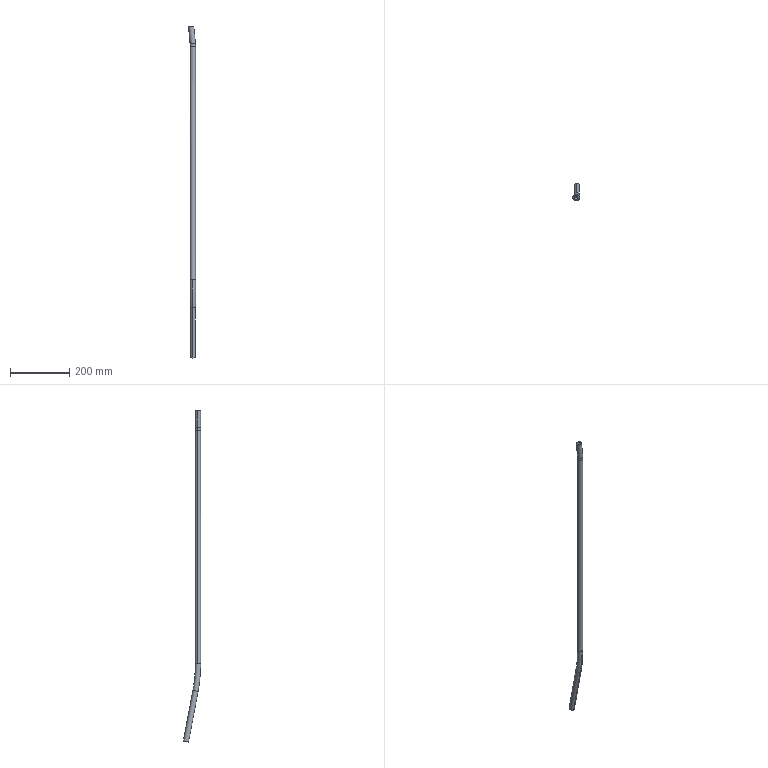Part | STEP file | Lower Chain Tube | 1 solid | 22 faces | box 23.853 x 58.527 x 1125 mm | volume 60168 mm3 | cylinder 12 | torus 8 | plane 2 | commonest cylinder face diameters 16 x6 18 x6
STEP:
#1=CARTESIAN_POINT('',(0.,0.,0.));
#2=DIRECTION('',(0.,0.,1.));
#3=DIRECTION('',(1.,0.,0.));
#4=AXIS2_PLACEMENT_3D('',#1,#2,#3);
#5=CARTESIAN_POINT('',(-8.,0.,3.704));
#6=VERTEX_POINT('',#5);
#7=CARTESIAN_POINT('',(-8.41,0.,12.377));
#8=VERTEX_POINT('',#7);
#9=CARTESIAN_POINT('',(-100.,0.,3.704));
#10=DIRECTION('',(0.,-1.,0.));
#11=DIRECTION('',(0.,0.,-1.));
#12=AXIS2_PLACEMENT_3D('',#9,#10,#11);
#13=CIRCLE('',#12,92.);
#14=CARTESIAN_POINT('',(-100.,0.,3.704));
#15=DIRECTION('',(0.,-1.,0.));
#16=DIRECTION('',(0.,0.,-1.));
#17=AXIS2_PLACEMENT_3D('',#14,#15,#16);
#18=TOROIDAL_SURFACE('',#17,100.,8.);
#19=CARTESIAN_POINT('',(0.,3.142));
#20=DIRECTION('',(1.,0.));
#21=VECTOR('',#20,1.);
#22=LINE('',#19,#21);
#23=(GEOMETRIC_REPRESENTATION_CONTEXT(2)PARAMETRIC_REPRESENTATION_CONTEXT()REPRESENTATION_CONTEXT('',''));
#24=DEFINITIONAL_REPRESENTATION('',(#22),#23);
#25=PCURVE('',#18,#24);
#26=CARTESIAN_POINT('',(-100.,0.,3.704));
#27=DIRECTION('',(0.,-1.,0.));
#28=DIRECTION('',(0.,0.,-1.));
#29=AXIS2_PLACEMENT_3D('',#26,#27,#28);
#30=TOROIDAL_SURFACE('',#29,100.,8.);
#31=CARTESIAN_POINT('',(0.,3.142));
#32=DIRECTION('',(1.,0.));
#33=VECTOR('',#32,1.);
#34=LINE('',#31,#33);
#35=(GEOMETRIC_REPRESENTATION_CONTEXT(2)PARAMETRIC_REPRESENTATION_CONTEXT()REPRESENTATION_CONTEXT('',''));
#36=DEFINITIONAL_REPRESENTATION('',(#34),#35);
#37=PCURVE('',#30,#36);
#38=SURFACE_CURVE('',#13,(#25,#37),.PCURVE_S1.);
#39=EDGE_CURVE('',#6,#8,#38,.T.);
#40=ORIENTED_EDGE('',*,*,#39,.T.);
#41=CARTESIAN_POINT('',(7.519,0.,13.885));
#42=VERTEX_POINT('',#41);
#43=CARTESIAN_POINT('',(-0.4454,0.,13.131));
#44=DIRECTION('',(-0.09427,0.,0.9955));
#45=DIRECTION('',(0.9955,0.,0.09427));
#46=AXIS2_PLACEMENT_3D('',#43,#44,#45);
#47=CIRCLE('',#46,8.);
#48=CARTESIAN_POINT('',(1.665,6.283));
#49=DIRECTION('',(0.,-1.));
#50=VECTOR('',#49,1.);
#51=LINE('',#48,#50);
#52=(GEOMETRIC_REPRESENTATION_CONTEXT(2)PARAMETRIC_REPRESENTATION_CONTEXT()REPRESENTATION_CONTEXT('',''));
#53=DEFINITIONAL_REPRESENTATION('',(#51),#52);
#54=PCURVE('',#18,#53);
#55=CARTESIAN_POINT('',(-0.4454,0.,13.131));
#56=DIRECTION('',(-0.09427,0.,0.9955));
#57=DIRECTION('',(0.9955,0.,0.09427));
#58=AXIS2_PLACEMENT_3D('',#55,#56,#57);
#59=CYLINDRICAL_SURFACE('',#58,8.);
#60=CARTESIAN_POINT('',(0.,0.));
#61=DIRECTION('',(1.,0.));
#62=VECTOR('',#61,1.);
#63=LINE('',#60,#62);
#64=(GEOMETRIC_REPRESENTATION_CONTEXT(2)PARAMETRIC_REPRESENTATION_CONTEXT()REPRESENTATION_CONTEXT('',''));
#65=DEFINITIONAL_REPRESENTATION('',(#63),#64);
#66=PCURVE('',#59,#65);
#67=SURFACE_CURVE('',#47,(#54,#66),.PCURVE_S1.);
#68=EDGE_CURVE('',#42,#8,#67,.T.);
#69=ORIENTED_EDGE('',*,*,#68,.F.);
#70=CARTESIAN_POINT('',(8.,0.,3.704));
#71=VERTEX_POINT('',#70);
#72=CARTESIAN_POINT('',(-100.,0.,3.704));
#73=DIRECTION('',(0.,-1.,0.));
#74=DIRECTION('',(0.,0.,-1.));
#75=AXIS2_PLACEMENT_3D('',#72,#73,#74);
#76=CIRCLE('',#75,108.);
#77=CARTESIAN_POINT('',(0.,6.283));
#78=DIRECTION('',(1.,0.));
#79=VECTOR('',#78,1.);
#80=LINE('',#77,#79);
#81=(GEOMETRIC_REPRESENTATION_CONTEXT(2)PARAMETRIC_REPRESENTATION_CONTEXT()REPRESENTATION_CONTEXT('',''));
#82=DEFINITIONAL_REPRESENTATION('',(#80),#81);
#83=PCURVE('',#18,#82);
#84=CARTESIAN_POINT('',(0.,0.));
#85=DIRECTION('',(1.,0.));
#86=VECTOR('',#85,1.);
#87=LINE('',#84,#86);
#88=(GEOMETRIC_REPRESENTATION_CONTEXT(2)PARAMETRIC_REPRESENTATION_CONTEXT()REPRESENTATION_CONTEXT('',''));
#89=DEFINITIONAL_REPRESENTATION('',(#87),#88);
#90=PCURVE('',#30,#89);
#91=SURFACE_CURVE('',#76,(#83,#90),.PCURVE_S1.);
#92=EDGE_CURVE('',#71,#42,#91,.T.);
#93=ORIENTED_EDGE('',*,*,#92,.F.);
#94=CARTESIAN_POINT('',(0.,0.,3.704));
#95=DIRECTION('',(0.,0.,1.));
#96=DIRECTION('',(1.,0.,0.));
#97=AXIS2_PLACEMENT_3D('',#94,#95,#96);
#98=CIRCLE('',#97,8.);
#99=CARTESIAN_POINT('',(1.571,6.283));
#100=DIRECTION('',(0.,-1.));
#101=VECTOR('',#100,1.);
#102=LINE('',#99,#101);
#103=(GEOMETRIC_REPRESENTATION_CONTEXT(2)PARAMETRIC_REPRESENTATION_CONTEXT()REPRESENTATION_CONTEXT('',''));
#104=DEFINITIONAL_REPRESENTATION('',(#102),#103);
#105=PCURVE('',#18,#104);
#106=CARTESIAN_POINT('',(0.,0.,-788.57));
#107=DIRECTION('',(0.,0.,1.));
#108=DIRECTION('',(1.,0.,0.));
#109=AXIS2_PLACEMENT_3D('',#106,#107,#108);
#110=CYLINDRICAL_SURFACE('',#109,8.);
#111=CARTESIAN_POINT('',(0.,792.273));
#112=DIRECTION('',(1.,0.));
#113=VECTOR('',#112,1.);
#114=LINE('',#111,#113);
#115=(GEOMETRIC_REPRESENTATION_CONTEXT(2)PARAMETRIC_REPRESENTATION_CONTEXT()REPRESENTATION_CONTEXT('',''));
#116=DEFINITIONAL_REPRESENTATION('',(#114),#115);
#117=PCURVE('',#110,#116);
#118=SURFACE_CURVE('',#98,(#105,#117),.PCURVE_S1.);
#119=EDGE_CURVE('',#71,#6,#118,.T.);
#120=ORIENTED_EDGE('',*,*,#119,.T.);
#121=EDGE_LOOP('',(#40,#69,#93,#120));
#122=FACE_BOUND('',#121,.F.);
#123=ADVANCED_FACE('',(#122),#18,.F.);
#124=CARTESIAN_POINT('',(-9.,0.,3.704));
#125=VERTEX_POINT('',#124);
#126=CARTESIAN_POINT('',(9.,0.,3.704));
#127=VERTEX_POINT('',#126);
#128=CARTESIAN_POINT('',(0.,0.,3.704));
#129=DIRECTION('',(0.,0.,1.));
#130=DIRECTION('',(1.,0.,0.));
#131=AXIS2_PLACEMENT_3D('',#128,#129,#130);
#132=CIRCLE('',#131,9.);
#133=CARTESIAN_POINT('',(-100.,0.,3.704));
#134=DIRECTION('',(0.,-1.,0.));
#135=DIRECTION('',(0.,0.,-1.));
#136=AXIS2_PLACEMENT_3D('',#133,#134,#135);
#137=TOROIDAL_SURFACE('',#136,100.,9.);
#138=CARTESIAN_POINT('',(1.571,6.283));
#139=DIRECTION('',(0.,-1.));
#140=VECTOR('',#139,1.);
#141=LINE('',#138,#140);
#142=(GEOMETRIC_REPRESENTATION_CONTEXT(2)PARAMETRIC_REPRESENTATION_CONTEXT()REPRESENTATION_CONTEXT('',''));
#143=DEFINITIONAL_REPRESENTATION('',(#141),#142);
#144=PCURVE('',#137,#143);
#145=CARTESIAN_POINT('',(0.,0.,-788.57));
#146=DIRECTION('',(0.,0.,1.));
#147=DIRECTION('',(1.,0.,0.));
#148=AXIS2_PLACEMENT_3D('',#145,#146,#147);
#149=CYLINDRICAL_SURFACE('',#148,9.);
#150=CARTESIAN_POINT('',(0.,792.273));
#151=DIRECTION('',(1.,0.));
#152=VECTOR('',#151,1.);
#153=LINE('',#150,#152);
#154=(GEOMETRIC_REPRESENTATION_CONTEXT(2)PARAMETRIC_REPRESENTATION_CONTEXT()REPRESENTATION_CONTEXT('',''));
#155=DEFINITIONAL_REPRESENTATION('',(#153),#154);
#156=PCURVE('',#149,#155);
#157=SURFACE_CURVE('',#132,(#144,#156),.PCURVE_S1.);
#158=EDGE_CURVE('',#125,#127,#157,.T.);
#159=ORIENTED_EDGE('',*,*,#158,.T.);
#160=CARTESIAN_POINT('',(8.515,0.,13.979));
#161=VERTEX_POINT('',#160);
#162=CARTESIAN_POINT('',(-100.,0.,3.704));
#163=DIRECTION('',(0.,-1.,0.));
#164=DIRECTION('',(0.,0.,-1.));
#165=AXIS2_PLACEMENT_3D('',#162,#163,#164);
#166=CIRCLE('',#165,109.);
#167=CARTESIAN_POINT('',(0.,0.));
#168=DIRECTION('',(1.,0.));
#169=VECTOR('',#168,1.);
#170=LINE('',#167,#169);
#171=(GEOMETRIC_REPRESENTATION_CONTEXT(2)PARAMETRIC_REPRESENTATION_CONTEXT()REPRESENTATION_CONTEXT('',''));
#172=DEFINITIONAL_REPRESENTATION('',(#170),#171);
#173=PCURVE('',#137,#172);
#174=CARTESIAN_POINT('',(-100.,0.,3.704));
#175=DIRECTION('',(0.,-1.,0.));
#176=DIRECTION('',(0.,0.,-1.));
#177=AXIS2_PLACEMENT_3D('',#174,#175,#176);
#178=TOROIDAL_SURFACE('',#177,100.,9.);
#179=CARTESIAN_POINT('',(0.,6.283));
#180=DIRECTION('',(1.,0.));
#181=VECTOR('',#180,1.);
#182=LINE('',#179,#181);
#183=(GEOMETRIC_REPRESENTATION_CONTEXT(2)PARAMETRIC_REPRESENTATION_CONTEXT()REPRESENTATION_CONTEXT('',''));
#184=DEFINITIONAL_REPRESENTATION('',(#182),#183);
#185=PCURVE('',#178,#184);
#186=SURFACE_CURVE('',#166,(#173,#185),.PCURVE_S1.);
#187=EDGE_CURVE('',#127,#161,#186,.T.);
#188=ORIENTED_EDGE('',*,*,#187,.T.);
#189=CARTESIAN_POINT('',(-9.405,0.,12.283));
#190=VERTEX_POINT('',#189);
#191=CARTESIAN_POINT('',(-0.4454,0.,13.131));
#192=DIRECTION('',(-0.09427,0.,0.9955));
#193=DIRECTION('',(0.9955,0.,0.09427));
#194=AXIS2_PLACEMENT_3D('',#191,#192,#193);
#195=CIRCLE('',#194,9.);
#196=CARTESIAN_POINT('',(1.665,6.283));
#197=DIRECTION('',(0.,-1.));
#198=VECTOR('',#197,1.);
#199=LINE('',#196,#198);
#200=(GEOMETRIC_REPRESENTATION_CONTEXT(2)PARAMETRIC_REPRESENTATION_CONTEXT()REPRESENTATION_CONTEXT('',''));
#201=DEFINITIONAL_REPRESENTATION('',(#199),#200);
#202=PCURVE('',#137,#201);
#203=CARTESIAN_POINT('',(-0.4454,0.,13.131));
#204=DIRECTION('',(-0.09427,0.,0.9955));
#205=DIRECTION('',(0.9955,0.,0.09427));
#206=AXIS2_PLACEMENT_3D('',#203,#204,#205);
#207=CYLINDRICAL_SURFACE('',#206,9.);
#208=CARTESIAN_POINT('',(0.,0.));
#209=DIRECTION('',(1.,0.));
#210=VECTOR('',#209,1.);
#211=LINE('',#208,#210);
#212=(GEOMETRIC_REPRESENTATION_CONTEXT(2)PARAMETRIC_REPRESENTATION_CONTEXT()REPRESENTATION_CONTEXT('',''));
#213=DEFINITIONAL_REPRESENTATION('',(#211),#212);
#214=PCURVE('',#207,#213);
#215=SURFACE_CURVE('',#195,(#202,#214),.PCURVE_S1.);
#216=EDGE_CURVE('',#190,#161,#215,.T.);
#217=ORIENTED_EDGE('',*,*,#216,.F.);
#218=CARTESIAN_POINT('',(-100.,0.,3.704));
#219=DIRECTION('',(0.,-1.,0.));
#220=DIRECTION('',(0.,0.,-1.));
#221=AXIS2_PLACEMENT_3D('',#218,#219,#220);
#222=CIRCLE('',#221,91.);
#223=CARTESIAN_POINT('',(0.,3.142));
#224=DIRECTION('',(1.,0.));
#225=VECTOR('',#224,1.);
#226=LINE('',#223,#225);
#227=(GEOMETRIC_REPRESENTATION_CONTEXT(2)PARAMETRIC_REPRESENTATION_CONTEXT()REPRESENTATION_CONTEXT('',''));
#228=DEFINITIONAL_REPRESENTATION('',(#226),#227);
#229=PCURVE('',#137,#228);
#230=CARTESIAN_POINT('',(0.,3.142));
#231=DIRECTION('',(1.,0.));
#232=VECTOR('',#231,1.);
#233=LINE('',#230,#232);
#234=(GEOMETRIC_REPRESENTATION_CONTEXT(2)PARAMETRIC_REPRESENTATION_CONTEXT()REPRESENTATION_CONTEXT('',''));
#235=DEFINITIONAL_REPRESENTATION('',(#233),#234);
#236=PCURVE('',#178,#235);
#237=SURFACE_CURVE('',#222,(#229,#236),.PCURVE_S1.);
#238=EDGE_CURVE('',#125,#190,#237,.T.);
#239=ORIENTED_EDGE('',*,*,#238,.F.);
#240=EDGE_LOOP('',(#159,#188,#217,#239));
#241=FACE_BOUND('',#240,.T.);
#242=ADVANCED_FACE('',(#241),#137,.T.);
#243=CARTESIAN_POINT('',(0.,8.,-788.57));
#244=VERTEX_POINT('',#243);
#245=CARTESIAN_POINT('',(-8.,0.,-788.57));
#246=VERTEX_POINT('',#245);
#247=CARTESIAN_POINT('',(0.,0.,-788.57));
#248=DIRECTION('',(0.,0.,1.));
#249=DIRECTION('',(1.,0.,0.));
#250=AXIS2_PLACEMENT_3D('',#247,#248,#249);
#251=CIRCLE('',#250,8.);
#252=CARTESIAN_POINT('',(0.,500.,-788.57));
#253=DIRECTION('',(1.,0.,0.));
#254=DIRECTION('',(0.,0.,-1.));
#255=AXIS2_PLACEMENT_3D('',#252,#253,#254);
#256=TOROIDAL_SURFACE('',#255,500.,8.);
#257=CARTESIAN_POINT('',(4.712,1.571));
#258=DIRECTION('',(0.,1.));
#259=VECTOR('',#258,1.);
#260=LINE('',#257,#259);
#261=(GEOMETRIC_REPRESENTATION_CONTEXT(2)PARAMETRIC_REPRESENTATION_CONTEXT()REPRESENTATION_CONTEXT('',''));
#262=DEFINITIONAL_REPRESENTATION('',(#260),#261);
#263=PCURVE('',#256,#262);
#264=CARTESIAN_POINT('',(0.,0.));
#265=DIRECTION('',(1.,0.));
#266=VECTOR('',#265,1.);
#267=LINE('',#264,#266);
#268=(GEOMETRIC_REPRESENTATION_CONTEXT(2)PARAMETRIC_REPRESENTATION_CONTEXT()REPRESENTATION_CONTEXT('',''));
#269=DEFINITIONAL_REPRESENTATION('',(#267),#268);
#270=PCURVE('',#110,#269);
#271=SURFACE_CURVE('',#251,(#263,#270),.PCURVE_S1.);
#272=EDGE_CURVE('',#244,#246,#271,.T.);
#273=ORIENTED_EDGE('',*,*,#272,.F.);
#274=CARTESIAN_POINT('',(0.,16.413,-879.163));
#275=VERTEX_POINT('',#274);
#276=CARTESIAN_POINT('',(0.,500.,-788.57));
#277=DIRECTION('',(1.,0.,0.));
#278=DIRECTION('',(0.,0.,-1.));
#279=AXIS2_PLACEMENT_3D('',#276,#277,#278);
#280=CIRCLE('',#279,492.);
#281=CARTESIAN_POINT('',(0.,3.142));
#282=DIRECTION('',(1.,0.));
#283=VECTOR('',#282,1.);
#284=LINE('',#281,#283);
#285=(GEOMETRIC_REPRESENTATION_CONTEXT(2)PARAMETRIC_REPRESENTATION_CONTEXT()REPRESENTATION_CONTEXT('',''));
#286=DEFINITIONAL_REPRESENTATION('',(#284),#285);
#287=PCURVE('',#256,#286);
#288=CARTESIAN_POINT('',(0.,500.,-788.57));
#289=DIRECTION('',(1.,0.,0.));
#290=DIRECTION('',(0.,0.,-1.));
#291=AXIS2_PLACEMENT_3D('',#288,#289,#290);
#292=TOROIDAL_SURFACE('',#291,500.,8.);
#293=CARTESIAN_POINT('',(0.,3.142));
#294=DIRECTION('',(1.,0.));
#295=VECTOR('',#294,1.);
#296=LINE('',#293,#295);
#297=(GEOMETRIC_REPRESENTATION_CONTEXT(2)PARAMETRIC_REPRESENTATION_CONTEXT()REPRESENTATION_CONTEXT('',''));
#298=DEFINITIONAL_REPRESENTATION('',(#296),#297);
#299=PCURVE('',#292,#298);
#300=SURFACE_CURVE('',#280,(#287,#299),.PCURVE_S1.);
#301=EDGE_CURVE('',#244,#275,#300,.T.);
#302=ORIENTED_EDGE('',*,*,#301,.T.);
#303=CARTESIAN_POINT('',(0.,0.6862,-882.11));
#304=VERTEX_POINT('',#303);
#305=CARTESIAN_POINT('',(0.,8.549,-880.637));
#306=DIRECTION('',(0.,-0.1841,0.9829));
#307=DIRECTION('',(1.,0.,0.));
#308=AXIS2_PLACEMENT_3D('',#305,#306,#307);
#309=CIRCLE('',#308,8.);
#310=CARTESIAN_POINT('',(4.898,1.571));
#311=DIRECTION('',(0.,1.));
#312=VECTOR('',#311,1.);
#313=LINE('',#310,#312);
#314=(GEOMETRIC_REPRESENTATION_CONTEXT(2)PARAMETRIC_REPRESENTATION_CONTEXT()REPRESENTATION_CONTEXT('',''));
#315=DEFINITIONAL_REPRESENTATION('',(#313),#314);
#316=PCURVE('',#256,#315);
#317=CARTESIAN_POINT('',(0.,8.549,-880.637));
#318=DIRECTION('',(0.,0.1841,-0.9829));
#319=DIRECTION('',(0.,0.9829,0.1841));
#320=AXIS2_PLACEMENT_3D('',#317,#318,#319);
#321=CYLINDRICAL_SURFACE('',#320,8.);
#322=CARTESIAN_POINT('',(7.854,0.));
#323=DIRECTION('',(-1.,0.));
#324=VECTOR('',#323,1.);
#325=LINE('',#322,#324);
#326=(GEOMETRIC_REPRESENTATION_CONTEXT(2)PARAMETRIC_REPRESENTATION_CONTEXT()REPRESENTATION_CONTEXT('',''));
#327=DEFINITIONAL_REPRESENTATION('',(#325),#326);
#328=PCURVE('',#321,#327);
#329=SURFACE_CURVE('',#309,(#316,#328),.PCURVE_S1.);
#330=EDGE_CURVE('',#275,#304,#329,.T.);
#331=ORIENTED_EDGE('',*,*,#330,.T.);
#332=CARTESIAN_POINT('',(0.,-8.,-788.57));
#333=VERTEX_POINT('',#332);
#334=CARTESIAN_POINT('',(0.,500.,-788.57));
#335=DIRECTION('',(1.,0.,0.));
#336=DIRECTION('',(0.,0.,-1.));
#337=AXIS2_PLACEMENT_3D('',#334,#335,#336);
#338=CIRCLE('',#337,508.);
#339=CARTESIAN_POINT('',(0.,6.283));
#340=DIRECTION('',(1.,0.));
#341=VECTOR('',#340,1.);
#342=LINE('',#339,#341);
#343=(GEOMETRIC_REPRESENTATION_CONTEXT(2)PARAMETRIC_REPRESENTATION_CONTEXT()REPRESENTATION_CONTEXT('',''));
#344=DEFINITIONAL_REPRESENTATION('',(#342),#343);
#345=PCURVE('',#256,#344);
#346=CARTESIAN_POINT('',(0.,0.));
#347=DIRECTION('',(1.,0.));
#348=VECTOR('',#347,1.);
#349=LINE('',#346,#348);
#350=(GEOMETRIC_REPRESENTATION_CONTEXT(2)PARAMETRIC_REPRESENTATION_CONTEXT()REPRESENTATION_CONTEXT('',''));
#351=DEFINITIONAL_REPRESENTATION('',(#349),#350);
#352=PCURVE('',#292,#351);
#353=SURFACE_CURVE('',#338,(#345,#352),.PCURVE_S1.);
#354=EDGE_CURVE('',#333,#304,#353,.T.);
#355=ORIENTED_EDGE('',*,*,#354,.F.);
#356=CARTESIAN_POINT('',(0.,0.,-788.57));
#357=DIRECTION('',(0.,0.,1.));
#358=DIRECTION('',(1.,0.,0.));
#359=AXIS2_PLACEMENT_3D('',#356,#357,#358);
#360=CIRCLE('',#359,8.);
#361=CARTESIAN_POINT('',(4.712,1.571));
#362=DIRECTION('',(0.,1.));
#363=VECTOR('',#362,1.);
#364=LINE('',#361,#363);
#365=(GEOMETRIC_REPRESENTATION_CONTEXT(2)PARAMETRIC_REPRESENTATION_CONTEXT()REPRESENTATION_CONTEXT('',''));
#366=DEFINITIONAL_REPRESENTATION('',(#364),#365);
#367=PCURVE('',#256,#366);
#368=CARTESIAN_POINT('',(0.,0.,-788.57));
#369=DIRECTION('',(0.,0.,1.));
#370=DIRECTION('',(1.,0.,0.));
#371=AXIS2_PLACEMENT_3D('',#368,#369,#370);
#372=CYLINDRICAL_SURFACE('',#371,8.);
#373=CARTESIAN_POINT('',(0.,0.));
#374=DIRECTION('',(1.,0.));
#375=VECTOR('',#374,1.);
#376=LINE('',#373,#375);
#377=(GEOMETRIC_REPRESENTATION_CONTEXT(2)PARAMETRIC_REPRESENTATION_CONTEXT()REPRESENTATION_CONTEXT('',''));
#378=DEFINITIONAL_REPRESENTATION('',(#376),#377);
#379=PCURVE('',#372,#378);
#380=SURFACE_CURVE('',#360,(#367,#379),.PCURVE_S1.);
#381=EDGE_CURVE('',#246,#333,#380,.T.);
#382=ORIENTED_EDGE('',*,*,#381,.F.);
#383=EDGE_LOOP('',(#273,#302,#331,#355,#382));
#384=FACE_BOUND('',#383,.F.);
#385=ADVANCED_FACE('',(#384),#256,.F.);
#386=CARTESIAN_POINT('',(0.,-9.,-788.57));
#387=VERTEX_POINT('',#386);
#388=CARTESIAN_POINT('',(9.,0.,-788.57));
#389=VERTEX_POINT('',#388);
#390=CARTESIAN_POINT('',(0.,0.,-788.57));
#391=DIRECTION('',(0.,0.,1.));
#392=DIRECTION('',(1.,0.,0.));
#393=AXIS2_PLACEMENT_3D('',#390,#391,#392);
#394=CIRCLE('',#393,9.);
#395=CARTESIAN_POINT('',(0.,500.,-788.57));
#396=DIRECTION('',(1.,0.,0.));
#397=DIRECTION('',(0.,0.,-1.));
#398=AXIS2_PLACEMENT_3D('',#395,#396,#397);
#399=TOROIDAL_SURFACE('',#398,500.,9.);
#400=CARTESIAN_POINT('',(4.712,-4.712));
#401=DIRECTION('',(0.,1.));
#402=VECTOR('',#401,1.);
#403=LINE('',#400,#402);
#404=(GEOMETRIC_REPRESENTATION_CONTEXT(2)PARAMETRIC_REPRESENTATION_CONTEXT()REPRESENTATION_CONTEXT('',''));
#405=DEFINITIONAL_REPRESENTATION('',(#403),#404);
#406=PCURVE('',#399,#405);
#407=CARTESIAN_POINT('',(0.,0.));
#408=DIRECTION('',(1.,0.));
#409=VECTOR('',#408,1.);
#410=LINE('',#407,#409);
#411=(GEOMETRIC_REPRESENTATION_CONTEXT(2)PARAMETRIC_REPRESENTATION_CONTEXT()REPRESENTATION_CONTEXT('',''));
#412=DEFINITIONAL_REPRESENTATION('',(#410),#411);
#413=PCURVE('',#149,#412);
#414=SURFACE_CURVE('',#394,(#406,#413),.PCURVE_S1.);
#415=EDGE_CURVE('',#387,#389,#414,.T.);
#416=ORIENTED_EDGE('',*,*,#415,.F.);
#417=CARTESIAN_POINT('',(0.,-0.2967,-882.294));
#418=VERTEX_POINT('',#417);
#419=CARTESIAN_POINT('',(0.,500.,-788.57));
#420=DIRECTION('',(1.,0.,0.));
#421=DIRECTION('',(0.,0.,-1.));
#422=AXIS2_PLACEMENT_3D('',#419,#420,#421);
#423=CIRCLE('',#422,509.);
#424=CARTESIAN_POINT('',(0.,0.));
#425=DIRECTION('',(1.,0.));
#426=VECTOR('',#425,1.);
#427=LINE('',#424,#426);
#428=(GEOMETRIC_REPRESENTATION_CONTEXT(2)PARAMETRIC_REPRESENTATION_CONTEXT()REPRESENTATION_CONTEXT('',''));
#429=DEFINITIONAL_REPRESENTATION('',(#427),#428);
#430=PCURVE('',#399,#429);
#431=CARTESIAN_POINT('',(0.,500.,-788.57));
#432=DIRECTION('',(1.,0.,0.));
#433=DIRECTION('',(0.,0.,-1.));
#434=AXIS2_PLACEMENT_3D('',#431,#432,#433);
#435=TOROIDAL_SURFACE('',#434,500.,9.);
#436=CARTESIAN_POINT('',(0.,6.283));
#437=DIRECTION('',(1.,0.));
#438=VECTOR('',#437,1.);
#439=LINE('',#436,#438);
#440=(GEOMETRIC_REPRESENTATION_CONTEXT(2)PARAMETRIC_REPRESENTATION_CONTEXT()REPRESENTATION_CONTEXT('',''));
#441=DEFINITIONAL_REPRESENTATION('',(#439),#440);
#442=PCURVE('',#435,#441);
#443=SURFACE_CURVE('',#423,(#430,#442),.PCURVE_S1.);
#444=EDGE_CURVE('',#387,#418,#443,.T.);
#445=ORIENTED_EDGE('',*,*,#444,.T.);
#446=CARTESIAN_POINT('',(0.,17.396,-878.979));
#447=VERTEX_POINT('',#446);
#448=CARTESIAN_POINT('',(0.,8.549,-880.637));
#449=DIRECTION('',(0.,-0.1841,0.9829));
#450=DIRECTION('',(1.,0.,0.));
#451=AXIS2_PLACEMENT_3D('',#448,#449,#450);
#452=CIRCLE('',#451,9.);
#453=CARTESIAN_POINT('',(4.898,-4.712));
#454=DIRECTION('',(0.,1.));
#455=VECTOR('',#454,1.);
#456=LINE('',#453,#455);
#457=(GEOMETRIC_REPRESENTATION_CONTEXT(2)PARAMETRIC_REPRESENTATION_CONTEXT()REPRESENTATION_CONTEXT('',''));
#458=DEFINITIONAL_REPRESENTATION('',(#456),#457);
#459=PCURVE('',#399,#458);
#460=CARTESIAN_POINT('',(0.,8.549,-880.637));
#461=DIRECTION('',(0.,0.1841,-0.9829));
#462=DIRECTION('',(0.,0.9829,0.1841));
#463=AXIS2_PLACEMENT_3D('',#460,#461,#462);
#464=CYLINDRICAL_SURFACE('',#463,9.);
#465=CARTESIAN_POINT('',(7.854,0.));
#466=DIRECTION('',(-1.,0.));
#467=VECTOR('',#466,1.);
#468=LINE('',#465,#467);
#469=(GEOMETRIC_REPRESENTATION_CONTEXT(2)PARAMETRIC_REPRESENTATION_CONTEXT()REPRESENTATION_CONTEXT('',''));
#470=DEFINITIONAL_REPRESENTATION('',(#468),#469);
#471=PCURVE('',#464,#470);
#472=SURFACE_CURVE('',#452,(#459,#471),.PCURVE_S1.);
#473=EDGE_CURVE('',#418,#447,#472,.T.);
#474=ORIENTED_EDGE('',*,*,#473,.T.);
#475=CARTESIAN_POINT('',(0.,9.,-788.57));
#476=VERTEX_POINT('',#475);
#477=CARTESIAN_POINT('',(0.,500.,-788.57));
#478=DIRECTION('',(1.,0.,0.));
#479=DIRECTION('',(0.,0.,-1.));
#480=AXIS2_PLACEMENT_3D('',#477,#478,#479);
#481=CIRCLE('',#480,491.);
#482=CARTESIAN_POINT('',(0.,3.142));
#483=DIRECTION('',(1.,0.));
#484=VECTOR('',#483,1.);
#485=LINE('',#482,#484);
#486=(GEOMETRIC_REPRESENTATION_CONTEXT(2)PARAMETRIC_REPRESENTATION_CONTEXT()REPRESENTATION_CONTEXT('',''));
#487=DEFINITIONAL_REPRESENTATION('',(#485),#486);
#488=PCURVE('',#399,#487);
#489=CARTESIAN_POINT('',(0.,3.142));
#490=DIRECTION('',(1.,0.));
#491=VECTOR('',#490,1.);
#492=LINE('',#489,#491);
#493=(GEOMETRIC_REPRESENTATION_CONTEXT(2)PARAMETRIC_REPRESENTATION_CONTEXT()REPRESENTATION_CONTEXT('',''));
#494=DEFINITIONAL_REPRESENTATION('',(#492),#493);
#495=PCURVE('',#435,#494);
#496=SURFACE_CURVE('',#481,(#488,#495),.PCURVE_S1.);
#497=EDGE_CURVE('',#476,#447,#496,.T.);
#498=ORIENTED_EDGE('',*,*,#497,.F.);
#499=CARTESIAN_POINT('',(0.,0.,-788.57));
#500=DIRECTION('',(0.,0.,1.));
#501=DIRECTION('',(1.,0.,0.));
#502=AXIS2_PLACEMENT_3D('',#499,#500,#501);
#503=CIRCLE('',#502,9.);
#504=CARTESIAN_POINT('',(4.712,1.571));
#505=DIRECTION('',(0.,1.));
#506=VECTOR('',#505,1.);
#507=LINE('',#504,#506);
#508=(GEOMETRIC_REPRESENTATION_CONTEXT(2)PARAMETRIC_REPRESENTATION_CONTEXT()REPRESENTATION_CONTEXT('',''));
#509=DEFINITIONAL_REPRESENTATION('',(#507),#508);
#510=PCURVE('',#399,#509);
#511=CARTESIAN_POINT('',(0.,0.,-788.57));
#512=DIRECTION('',(0.,0.,1.));
#513=DIRECTION('',(1.,0.,0.));
#514=AXIS2_PLACEMENT_3D('',#511,#512,#513);
#515=CYLINDRICAL_SURFACE('',#514,9.);
#516=CARTESIAN_POINT('',(0.,0.));
#517=DIRECTION('',(1.,0.));
#518=VECTOR('',#517,1.);
#519=LINE('',#516,#518);
#520=(GEOMETRIC_REPRESENTATION_CONTEXT(2)PARAMETRIC_REPRESENTATION_CONTEXT()REPRESENTATION_CONTEXT('',''));
#521=DEFINITIONAL_REPRESENTATION('',(#519),#520);
#522=PCURVE('',#515,#521);
#523=SURFACE_CURVE('',#503,(#510,#522),.PCURVE_S1.);
#524=EDGE_CURVE('',#389,#476,#523,.T.);
#525=ORIENTED_EDGE('',*,*,#524,.F.);
#526=EDGE_LOOP('',(#416,#445,#474,#498,#525));
#527=FACE_BOUND('',#526,.T.);
#528=ADVANCED_FACE('',(#527),#399,.T.);
#529=CARTESIAN_POINT('',(2.071,0.,71.416));
#530=VERTEX_POINT('',#529);
#531=CARTESIAN_POINT('',(7.519,0.,13.885));
#532=DIRECTION('',(-0.09427,0.,0.9955));
#533=VECTOR('',#532,1.);
#534=LINE('',#531,#533);
#535=CARTESIAN_POINT('',(-0.4454,0.,13.131));
#536=DIRECTION('',(-0.09427,0.,0.9955));
#537=DIRECTION('',(0.9955,0.,0.09427));
#538=AXIS2_PLACEMENT_3D('',#535,#536,#537);
#539=CYLINDRICAL_SURFACE('',#538,8.);
#540=CARTESIAN_POINT('',(6.283,0.));
#541=DIRECTION('',(0.,1.));
#542=VECTOR('',#541,1.);
#543=LINE('',#540,#542);
#544=(GEOMETRIC_REPRESENTATION_CONTEXT(2)PARAMETRIC_REPRESENTATION_CONTEXT()REPRESENTATION_CONTEXT('',''));
#545=DEFINITIONAL_REPRESENTATION('',(#543),#544);
#546=PCURVE('',#539,#545);
#547=CARTESIAN_POINT('',(0.,0.));
#548=DIRECTION('',(0.,1.));
#549=VECTOR('',#548,1.);
#550=LINE('',#547,#549);
#551=(GEOMETRIC_REPRESENTATION_CONTEXT(2)PARAMETRIC_REPRESENTATION_CONTEXT()REPRESENTATION_CONTEXT('',''));
#552=DEFINITIONAL_REPRESENTATION('',(#550),#551);
#553=PCURVE('',#59,#552);
#554=SURFACE_CURVE('',#534,(#546,#553),.PCURVE_S1.);
#555=EDGE_CURVE('',#42,#530,#554,.T.);
#556=ORIENTED_EDGE('',*,*,#555,.T.);
#557=CARTESIAN_POINT('',(-13.858,0.,69.908));
#558=VERTEX_POINT('',#557);
#559=CARTESIAN_POINT('',(-5.893,0.,70.662));
#560=DIRECTION('',(-0.09427,0.,0.9955));
#561=DIRECTION('',(0.9955,0.,0.09427));
#562=AXIS2_PLACEMENT_3D('',#559,#560,#561);
#563=CIRCLE('',#562,8.);
#564=CARTESIAN_POINT('',(0.,57.788));
#565=DIRECTION('',(1.,0.));
#566=VECTOR('',#565,1.);
#567=LINE('',#564,#566);
#568=(GEOMETRIC_REPRESENTATION_CONTEXT(2)PARAMETRIC_REPRESENTATION_CONTEXT()REPRESENTATION_CONTEXT('',''));
#569=DEFINITIONAL_REPRESENTATION('',(#567),#568);
#570=PCURVE('',#539,#569);
#571=CARTESIAN_POINT('',(-5.893,0.,70.662));
#572=DIRECTION('',(-0.09427,0.,0.9955));
#573=DIRECTION('',(0.9955,0.,0.09427));
#574=AXIS2_PLACEMENT_3D('',#571,#572,#573);
#575=PLANE('',#574);
#576=CARTESIAN_POINT('',(0.,0.));
#577=DIRECTION('',(1.,0.));
#578=AXIS2_PLACEMENT_2D('',#576,#577);
#579=CIRCLE('',#578,8.);
#580=(GEOMETRIC_REPRESENTATION_CONTEXT(2)PARAMETRIC_REPRESENTATION_CONTEXT()REPRESENTATION_CONTEXT('',''));
#581=DEFINITIONAL_REPRESENTATION('',(#579),#580);
#582=PCURVE('',#575,#581);
#583=SURFACE_CURVE('',#563,(#570,#582),.PCURVE_S1.);
#584=EDGE_CURVE('',#558,#530,#583,.T.);
#585=ORIENTED_EDGE('',*,*,#584,.F.);
#586=CARTESIAN_POINT('',(-8.41,0.,12.377));
#587=DIRECTION('',(-0.09427,0.,0.9955));
#588=VECTOR('',#587,1.);
#589=LINE('',#586,#588);
#590=CARTESIAN_POINT('',(3.142,0.));
#591=DIRECTION('',(0.,1.));
#592=VECTOR('',#591,1.);
#593=LINE('',#590,#592);
#594=(GEOMETRIC_REPRESENTATION_CONTEXT(2)PARAMETRIC_REPRESENTATION_CONTEXT()REPRESENTATION_CONTEXT('',''));
#595=DEFINITIONAL_REPRESENTATION('',(#593),#594);
#596=PCURVE('',#539,#595);
#597=CARTESIAN_POINT('',(3.142,0.));
#598=DIRECTION('',(0.,1.));
#599=VECTOR('',#598,1.);
#600=LINE('',#597,#599);
#601=(GEOMETRIC_REPRESENTATION_CONTEXT(2)PARAMETRIC_REPRESENTATION_CONTEXT()REPRESENTATION_CONTEXT('',''));
#602=DEFINITIONAL_REPRESENTATION('',(#600),#601);
#603=PCURVE('',#59,#602);
#604=SURFACE_CURVE('',#589,(#596,#603),.PCURVE_S1.);
#605=EDGE_CURVE('',#8,#558,#604,.T.);
#606=ORIENTED_EDGE('',*,*,#605,.F.);
#607=CARTESIAN_POINT('',(-0.4454,0.,13.131));
#608=DIRECTION('',(-0.09427,0.,0.9955));
#609=DIRECTION('',(0.9955,0.,0.09427));
#610=AXIS2_PLACEMENT_3D('',#607,#608,#609);
#611=CIRCLE('',#610,8.);
#612=CARTESIAN_POINT('',(0.,0.));
#613=DIRECTION('',(1.,0.));
#614=VECTOR('',#613,1.);
#615=LINE('',#612,#614);
#616=(GEOMETRIC_REPRESENTATION_CONTEXT(2)PARAMETRIC_REPRESENTATION_CONTEXT()REPRESENTATION_CONTEXT('',''));
#617=DEFINITIONAL_REPRESENTATION('',(#615),#616);
#618=PCURVE('',#539,#617);
#619=CARTESIAN_POINT('',(1.665,6.283));
#620=DIRECTION('',(0.,-1.));
#621=VECTOR('',#620,1.);
#622=LINE('',#619,#621);
#623=(GEOMETRIC_REPRESENTATION_CONTEXT(2)PARAMETRIC_REPRESENTATION_CONTEXT()REPRESENTATION_CONTEXT('',''));
#624=DEFINITIONAL_REPRESENTATION('',(#622),#623);
#625=PCURVE('',#30,#624);
#626=SURFACE_CURVE('',#611,(#618,#625),.PCURVE_S1.);
#627=EDGE_CURVE('',#8,#42,#626,.T.);
#628=ORIENTED_EDGE('',*,*,#627,.T.);
#629=EDGE_LOOP('',(#556,#585,#606,#628));
#630=FACE_BOUND('',#629,.F.);
#631=ADVANCED_FACE('',(#630),#539,.F.);
#632=CARTESIAN_POINT('',(-0.4454,0.,13.131));
#633=DIRECTION('',(-0.09427,0.,0.9955));
#634=DIRECTION('',(0.9955,0.,0.09427));
#635=AXIS2_PLACEMENT_3D('',#632,#633,#634);
#636=CIRCLE('',#635,9.);
#637=CARTESIAN_POINT('',(-0.4454,0.,13.131));
#638=DIRECTION('',(-0.09427,0.,0.9955));
#639=DIRECTION('',(0.9955,0.,0.09427));
#640=AXIS2_PLACEMENT_3D('',#637,#638,#639);
#641=CYLINDRICAL_SURFACE('',#640,9.);
#642=CARTESIAN_POINT('',(0.,0.));
#643=DIRECTION('',(1.,0.));
#644=VECTOR('',#643,1.);
#645=LINE('',#642,#644);
#646=(GEOMETRIC_REPRESENTATION_CONTEXT(2)PARAMETRIC_REPRESENTATION_CONTEXT()REPRESENTATION_CONTEXT('',''));
#647=DEFINITIONAL_REPRESENTATION('',(#645),#646);
#648=PCURVE('',#641,#647);
#649=CARTESIAN_POINT('',(1.665,6.283));
#650=DIRECTION('',(0.,-1.));
#651=VECTOR('',#650,1.);
#652=LINE('',#649,#651);
#653=(GEOMETRIC_REPRESENTATION_CONTEXT(2)PARAMETRIC_REPRESENTATION_CONTEXT()REPRESENTATION_CONTEXT('',''));
#654=DEFINITIONAL_REPRESENTATION('',(#652),#653);
#655=PCURVE('',#178,#654);
#656=SURFACE_CURVE('',#636,(#648,#655),.PCURVE_S1.);
#657=EDGE_CURVE('',#161,#190,#656,.T.);
#658=ORIENTED_EDGE('',*,*,#657,.T.);
#659=CARTESIAN_POINT('',(-14.853,0.,69.813));
#660=VERTEX_POINT('',#659);
#661=CARTESIAN_POINT('',(-9.405,0.,12.283));
#662=DIRECTION('',(-0.09427,0.,0.9955));
#663=VECTOR('',#662,1.);
#664=LINE('',#661,#663);
#665=CARTESIAN_POINT('',(3.142,0.));
#666=DIRECTION('',(0.,1.));
#667=VECTOR('',#666,1.);
#668=LINE('',#665,#667);
#669=(GEOMETRIC_REPRESENTATION_CONTEXT(2)PARAMETRIC_REPRESENTATION_CONTEXT()REPRESENTATION_CONTEXT('',''));
#670=DEFINITIONAL_REPRESENTATION('',(#668),#669);
#671=PCURVE('',#641,#670);
#672=CARTESIAN_POINT('',(3.142,0.));
#673=DIRECTION('',(0.,1.));
#674=VECTOR('',#673,1.);
#675=LINE('',#672,#674);
#676=(GEOMETRIC_REPRESENTATION_CONTEXT(2)PARAMETRIC_REPRESENTATION_CONTEXT()REPRESENTATION_CONTEXT('',''));
#677=DEFINITIONAL_REPRESENTATION('',(#675),#676);
#678=PCURVE('',#207,#677);
#679=SURFACE_CURVE('',#664,(#671,#678),.PCURVE_S1.);
#680=EDGE_CURVE('',#190,#660,#679,.T.);
#681=ORIENTED_EDGE('',*,*,#680,.T.);
#682=CARTESIAN_POINT('',(3.067,0.,71.51));
#683=VERTEX_POINT('',#682);
#684=CARTESIAN_POINT('',(-5.893,0.,70.662));
#685=DIRECTION('',(-0.09427,0.,0.9955));
#686=DIRECTION('',(0.9955,0.,0.09427));
#687=AXIS2_PLACEMENT_3D('',#684,#685,#686);
#688=CIRCLE('',#687,9.);
#689=CARTESIAN_POINT('',(0.,57.788));
#690=DIRECTION('',(1.,0.));
#691=VECTOR('',#690,1.);
#692=LINE('',#689,#691);
#693=(GEOMETRIC_REPRESENTATION_CONTEXT(2)PARAMETRIC_REPRESENTATION_CONTEXT()REPRESENTATION_CONTEXT('',''));
#694=DEFINITIONAL_REPRESENTATION('',(#692),#693);
#695=PCURVE('',#641,#694);
#696=CARTESIAN_POINT('',(0.,0.));
#697=DIRECTION('',(1.,0.));
#698=AXIS2_PLACEMENT_2D('',#696,#697);
#699=CIRCLE('',#698,9.);
#700=(GEOMETRIC_REPRESENTATION_CONTEXT(2)PARAMETRIC_REPRESENTATION_CONTEXT()REPRESENTATION_CONTEXT('',''));
#701=DEFINITIONAL_REPRESENTATION('',(#699),#700);
#702=PCURVE('',#575,#701);
#703=SURFACE_CURVE('',#688,(#695,#702),.PCURVE_S1.);
#704=EDGE_CURVE('',#683,#660,#703,.T.);
#705=ORIENTED_EDGE('',*,*,#704,.F.);
#706=CARTESIAN_POINT('',(8.515,0.,13.979));
#707=DIRECTION('',(-0.09427,0.,0.9955));
#708=VECTOR('',#707,1.);
#709=LINE('',#706,#708);
#710=CARTESIAN_POINT('',(0.,0.));
#711=DIRECTION('',(0.,1.));
#712=VECTOR('',#711,1.);
#713=LINE('',#710,#712);
#714=(GEOMETRIC_REPRESENTATION_CONTEXT(2)PARAMETRIC_REPRESENTATION_CONTEXT()REPRESENTATION_CONTEXT('',''));
#715=DEFINITIONAL_REPRESENTATION('',(#713),#714);
#716=PCURVE('',#641,#715);
#717=CARTESIAN_POINT('',(6.283,0.));
#718=DIRECTION('',(0.,1.));
#719=VECTOR('',#718,1.);
#720=LINE('',#717,#719);
#721=(GEOMETRIC_REPRESENTATION_CONTEXT(2)PARAMETRIC_REPRESENTATION_CONTEXT()REPRESENTATION_CONTEXT('',''));
#722=DEFINITIONAL_REPRESENTATION('',(#720),#721);
#723=PCURVE('',#207,#722);
#724=SURFACE_CURVE('',#709,(#716,#723),.PCURVE_S1.);
#725=EDGE_CURVE('',#161,#683,#724,.T.);
#726=ORIENTED_EDGE('',*,*,#725,.F.);
#727=EDGE_LOOP('',(#658,#681,#705,#726));
#728=FACE_BOUND('',#727,.T.);
#729=ADVANCED_FACE('',(#728),#641,.T.);
#730=ORIENTED_EDGE('',*,*,#524,.T.);
#731=CARTESIAN_POINT('',(-9.,0.,-788.57));
#732=VERTEX_POINT('',#731);
#733=CARTESIAN_POINT('',(0.,0.,-788.57));
#734=DIRECTION('',(0.,0.,1.));
#735=DIRECTION('',(1.,0.,0.));
#736=AXIS2_PLACEMENT_3D('',#733,#734,#735);
#737=CIRCLE('',#736,9.);
#738=CARTESIAN_POINT('',(0.,0.));
#739=DIRECTION('',(1.,0.));
#740=VECTOR('',#739,1.);
#741=LINE('',#738,#740);
#742=(GEOMETRIC_REPRESENTATION_CONTEXT(2)PARAMETRIC_REPRESENTATION_CONTEXT()REPRESENTATION_CONTEXT('',''));
#743=DEFINITIONAL_REPRESENTATION('',(#741),#742);
#744=PCURVE('',#515,#743);
#745=CARTESIAN_POINT('',(4.712,1.571));
#746=DIRECTION('',(0.,1.));
#747=VECTOR('',#746,1.);
#748=LINE('',#745,#747);
#749=(GEOMETRIC_REPRESENTATION_CONTEXT(2)PARAMETRIC_REPRESENTATION_CONTEXT()REPRESENTATION_CONTEXT('',''));
#750=DEFINITIONAL_REPRESENTATION('',(#748),#749);
#751=PCURVE('',#435,#750);
#752=SURFACE_CURVE('',#737,(#744,#751),.PCURVE_S1.);
#753=EDGE_CURVE('',#476,#732,#752,.T.);
#754=ORIENTED_EDGE('',*,*,#753,.T.);
#755=CARTESIAN_POINT('',(-9.,0.,-788.57));
#756=DIRECTION('',(0.,0.,1.));
#757=VECTOR('',#756,1.);
#758=LINE('',#755,#757);
#759=CARTESIAN_POINT('',(3.142,0.));
#760=DIRECTION('',(0.,1.));
#761=VECTOR('',#760,1.);
#762=LINE('',#759,#761);
#763=(GEOMETRIC_REPRESENTATION_CONTEXT(2)PARAMETRIC_REPRESENTATION_CONTEXT()REPRESENTATION_CONTEXT('',''));
#764=DEFINITIONAL_REPRESENTATION('',(#762),#763);
#765=PCURVE('',#515,#764);
#766=CARTESIAN_POINT('',(3.142,0.));
#767=DIRECTION('',(0.,1.));
#768=VECTOR('',#767,1.);
#769=LINE('',#766,#768);
#770=(GEOMETRIC_REPRESENTATION_CONTEXT(2)PARAMETRIC_REPRESENTATION_CONTEXT()REPRESENTATION_CONTEXT('',''));
#771=DEFINITIONAL_REPRESENTATION('',(#769),#770);
#772=PCURVE('',#149,#771);
#773=SURFACE_CURVE('',#758,(#765,#772),.PCURVE_S1.);
#774=EDGE_CURVE('',#732,#125,#773,.T.);
#775=ORIENTED_EDGE('',*,*,#774,.T.);
#776=CARTESIAN_POINT('',(0.,0.,3.704));
#777=DIRECTION('',(0.,0.,1.));
#778=DIRECTION('',(1.,0.,0.));
#779=AXIS2_PLACEMENT_3D('',#776,#777,#778);
#780=CIRCLE('',#779,9.);
#781=CARTESIAN_POINT('',(0.,792.273));
#782=DIRECTION('',(1.,0.));
#783=VECTOR('',#782,1.);
#784=LINE('',#781,#783);
#785=(GEOMETRIC_REPRESENTATION_CONTEXT(2)PARAMETRIC_REPRESENTATION_CONTEXT()REPRESENTATION_CONTEXT('',''));
#786=DEFINITIONAL_REPRESENTATION('',(#784),#785);
#787=PCURVE('',#515,#786);
#788=CARTESIAN_POINT('',(1.571,6.283));
#789=DIRECTION('',(0.,-1.));
#790=VECTOR('',#789,1.);
#791=LINE('',#788,#790);
#792=(GEOMETRIC_REPRESENTATION_CONTEXT(2)PARAMETRIC_REPRESENTATION_CONTEXT()REPRESENTATION_CONTEXT('',''));
#793=DEFINITIONAL_REPRESENTATION('',(#791),#792);
#794=PCURVE('',#178,#793);
#795=SURFACE_CURVE('',#780,(#787,#794),.PCURVE_S1.);
#796=EDGE_CURVE('',#127,#125,#795,.T.);
#797=ORIENTED_EDGE('',*,*,#796,.F.);
#798=CARTESIAN_POINT('',(9.,0.,-788.57));
#799=DIRECTION('',(0.,0.,1.));
#800=VECTOR('',#799,1.);
#801=LINE('',#798,#800);
#802=CARTESIAN_POINT('',(0.,0.));
#803=DIRECTION('',(0.,1.));
#804=VECTOR('',#803,1.);
#805=LINE('',#802,#804);
#806=(GEOMETRIC_REPRESENTATION_CONTEXT(2)PARAMETRIC_REPRESENTATION_CONTEXT()REPRESENTATION_CONTEXT('',''));
#807=DEFINITIONAL_REPRESENTATION('',(#805),#806);
#808=PCURVE('',#515,#807);
#809=CARTESIAN_POINT('',(6.283,0.));
#810=DIRECTION('',(0.,1.));
#811=VECTOR('',#810,1.);
#812=LINE('',#809,#811);
#813=(GEOMETRIC_REPRESENTATION_CONTEXT(2)PARAMETRIC_REPRESENTATION_CONTEXT()REPRESENTATION_CONTEXT('',''));
#814=DEFINITIONAL_REPRESENTATION('',(#812),#813);
#815=PCURVE('',#149,#814);
#816=SURFACE_CURVE('',#801,(#808,#815),.PCURVE_S1.);
#817=EDGE_CURVE('',#389,#127,#816,.T.);
#818=ORIENTED_EDGE('',*,*,#817,.F.);
#819=EDGE_LOOP('',(#730,#754,#775,#797,#818));
#820=FACE_BOUND('',#819,.T.);
#821=ADVANCED_FACE('',(#820),#515,.T.);
#822=CARTESIAN_POINT('',(8.,0.,-788.57));
#823=VERTEX_POINT('',#822);
#824=CARTESIAN_POINT('',(0.,0.,-788.57));
#825=DIRECTION('',(0.,0.,1.));
#826=DIRECTION('',(1.,0.,0.));
#827=AXIS2_PLACEMENT_3D('',#824,#825,#826);
#828=CIRCLE('',#827,8.);
#829=CARTESIAN_POINT('',(0.,0.));
#830=DIRECTION('',(1.,0.));
#831=VECTOR('',#830,1.);
#832=LINE('',#829,#831);
#833=(GEOMETRIC_REPRESENTATION_CONTEXT(2)PARAMETRIC_REPRESENTATION_CONTEXT()REPRESENTATION_CONTEXT('',''));
#834=DEFINITIONAL_REPRESENTATION('',(#832),#833);
#835=PCURVE('',#372,#834);
#836=CARTESIAN_POINT('',(4.712,-4.712));
#837=DIRECTION('',(0.,1.));
#838=VECTOR('',#837,1.);
#839=LINE('',#836,#838);
#840=(GEOMETRIC_REPRESENTATION_CONTEXT(2)PARAMETRIC_REPRESENTATION_CONTEXT()REPRESENTATION_CONTEXT('',''));
#841=DEFINITIONAL_REPRESENTATION('',(#839),#840);
#842=PCURVE('',#292,#841);
#843=SURFACE_CURVE('',#828,(#835,#842),.PCURVE_S1.);
#844=EDGE_CURVE('',#333,#823,#843,.T.);
#845=ORIENTED_EDGE('',*,*,#844,.T.);
#846=CARTESIAN_POINT('',(8.,0.,-788.57));
#847=DIRECTION('',(0.,0.,1.));
#848=VECTOR('',#847,1.);
#849=LINE('',#846,#848);
#850=CARTESIAN_POINT('',(6.283,0.));
#851=DIRECTION('',(0.,1.));
#852=VECTOR('',#851,1.);
#853=LINE('',#850,#852);
#854=(GEOMETRIC_REPRESENTATION_CONTEXT(2)PARAMETRIC_REPRESENTATION_CONTEXT()REPRESENTATION_CONTEXT('',''));
#855=DEFINITIONAL_REPRESENTATION('',(#853),#854);
#856=PCURVE('',#372,#855);
#857=CARTESIAN_POINT('',(0.,0.));
#858=DIRECTION('',(0.,1.));
#859=VECTOR('',#858,1.);
#860=LINE('',#857,#859);
#861=(GEOMETRIC_REPRESENTATION_CONTEXT(2)PARAMETRIC_REPRESENTATION_CONTEXT()REPRESENTATION_CONTEXT('',''));
#862=DEFINITIONAL_REPRESENTATION('',(#860),#861);
#863=PCURVE('',#110,#862);
#864=SURFACE_CURVE('',#849,(#856,#863),.PCURVE_S1.);
#865=EDGE_CURVE('',#823,#71,#864,.T.);
#866=ORIENTED_EDGE('',*,*,#865,.T.);
#867=CARTESIAN_POINT('',(0.,0.,3.704));
#868=DIRECTION('',(0.,0.,1.));
#869=DIRECTION('',(1.,0.,0.));
#870=AXIS2_PLACEMENT_3D('',#867,#868,#869);
#871=CIRCLE('',#870,8.);
#872=CARTESIAN_POINT('',(0.,792.273));
#873=DIRECTION('',(1.,0.));
#874=VECTOR('',#873,1.);
#875=LINE('',#872,#874);
#876=(GEOMETRIC_REPRESENTATION_CONTEXT(2)PARAMETRIC_REPRESENTATION_CONTEXT()REPRESENTATION_CONTEXT('',''));
#877=DEFINITIONAL_REPRESENTATION('',(#875),#876);
#878=PCURVE('',#372,#877);
#879=CARTESIAN_POINT('',(1.571,6.283));
#880=DIRECTION('',(0.,-1.));
#881=VECTOR('',#880,1.);
#882=LINE('',#879,#881);
#883=(GEOMETRIC_REPRESENTATION_CONTEXT(2)PARAMETRIC_REPRESENTATION_CONTEXT()REPRESENTATION_CONTEXT('',''));
#884=DEFINITIONAL_REPRESENTATION('',(#882),#883);
#885=PCURVE('',#30,#884);
#886=SURFACE_CURVE('',#871,(#878,#885),.PCURVE_S1.);
#887=EDGE_CURVE('',#6,#71,#886,.T.);
#888=ORIENTED_EDGE('',*,*,#887,.F.);
#889=CARTESIAN_POINT('',(-8.,0.,-788.57));
#890=DIRECTION('',(0.,0.,1.));
#891=VECTOR('',#890,1.);
#892=LINE('',#889,#891);
#893=CARTESIAN_POINT('',(3.142,0.));
#894=DIRECTION('',(0.,1.));
#895=VECTOR('',#894,1.);
#896=LINE('',#893,#895);
#897=(GEOMETRIC_REPRESENTATION_CONTEXT(2)PARAMETRIC_REPRESENTATION_CONTEXT()REPRESENTATION_CONTEXT('',''));
#898=DEFINITIONAL_REPRESENTATION('',(#896),#897);
#899=PCURVE('',#372,#898);
#900=CARTESIAN_POINT('',(3.142,0.));
#901=DIRECTION('',(0.,1.));
#902=VECTOR('',#901,1.);
#903=LINE('',#900,#902);
#904=(GEOMETRIC_REPRESENTATION_CONTEXT(2)PARAMETRIC_REPRESENTATION_CONTEXT()REPRESENTATION_CONTEXT('',''));
#905=DEFINITIONAL_REPRESENTATION('',(#903),#904);
#906=PCURVE('',#110,#905);
#907=SURFACE_CURVE('',#892,(#899,#906),.PCURVE_S1.);
#908=EDGE_CURVE('',#246,#6,#907,.T.);
#909=ORIENTED_EDGE('',*,*,#908,.F.);
#910=ORIENTED_EDGE('',*,*,#381,.T.);
#911=EDGE_LOOP('',(#845,#866,#888,#909,#910));
#912=FACE_BOUND('',#911,.F.);
#913=ADVANCED_FACE('',(#912),#372,.F.);
#914=CARTESIAN_POINT('',(0.,48.544,-1050.68));
#915=VERTEX_POINT('',#914);
#916=CARTESIAN_POINT('',(0.,16.413,-879.163));
#917=DIRECTION('',(0.,0.1841,-0.9829));
#918=VECTOR('',#917,1.);
#919=LINE('',#916,#918);
#920=CARTESIAN_POINT('',(6.283,0.));
#921=DIRECTION('',(0.,1.));
#922=VECTOR('',#921,1.);
#923=LINE('',#920,#922);
#924=(GEOMETRIC_REPRESENTATION_CONTEXT(2)PARAMETRIC_REPRESENTATION_CONTEXT()REPRESENTATION_CONTEXT('',''));
#925=DEFINITIONAL_REPRESENTATION('',(#923),#924);
#926=PCURVE('',#321,#925);
#927=CARTESIAN_POINT('',(0.,8.549,-880.637));
#928=DIRECTION('',(0.,0.1841,-0.9829));
#929=DIRECTION('',(0.,0.9829,0.1841));
#930=AXIS2_PLACEMENT_3D('',#927,#928,#929);
#931=CYLINDRICAL_SURFACE('',#930,8.);
#932=CARTESIAN_POINT('',(0.,0.));
#933=DIRECTION('',(0.,1.));
#934=VECTOR('',#933,1.);
#935=LINE('',#932,#934);
#936=(GEOMETRIC_REPRESENTATION_CONTEXT(2)PARAMETRIC_REPRESENTATION_CONTEXT()REPRESENTATION_CONTEXT('',''));
#937=DEFINITIONAL_REPRESENTATION('',(#935),#936);
#938=PCURVE('',#931,#937);
#939=SURFACE_CURVE('',#919,(#926,#938),.PCURVE_S1.);
#940=EDGE_CURVE('',#275,#915,#939,.T.);
#941=ORIENTED_EDGE('',*,*,#940,.T.);
#942=CARTESIAN_POINT('',(0.,32.818,-1053.627));
#943=VERTEX_POINT('',#942);
#944=CARTESIAN_POINT('',(0.,40.681,-1052.154));
#945=DIRECTION('',(0.,-0.1841,0.9829));
#946=DIRECTION('',(1.,0.,0.));
#947=AXIS2_PLACEMENT_3D('',#944,#945,#946);
#948=CIRCLE('',#947,8.);
#949=CARTESIAN_POINT('',(7.854,174.501));
#950=DIRECTION('',(-1.,0.));
#951=VECTOR('',#950,1.);
#952=LINE('',#949,#951);
#953=(GEOMETRIC_REPRESENTATION_CONTEXT(2)PARAMETRIC_REPRESENTATION_CONTEXT()REPRESENTATION_CONTEXT('',''));
#954=DEFINITIONAL_REPRESENTATION('',(#952),#953);
#955=PCURVE('',#321,#954);
#956=CARTESIAN_POINT('',(0.,40.681,-1052.154));
#957=DIRECTION('',(0.,-0.1841,0.9829));
#958=DIRECTION('',(1.,0.,0.));
#959=AXIS2_PLACEMENT_3D('',#956,#957,#958);
#960=PLANE('',#959);
#961=CARTESIAN_POINT('',(0.,0.));
#962=DIRECTION('',(1.,0.));
#963=AXIS2_PLACEMENT_2D('',#961,#962);
#964=CIRCLE('',#963,8.);
#965=(GEOMETRIC_REPRESENTATION_CONTEXT(2)PARAMETRIC_REPRESENTATION_CONTEXT()REPRESENTATION_CONTEXT('',''));
#966=DEFINITIONAL_REPRESENTATION('',(#964),#965);
#967=PCURVE('',#960,#966);
#968=SURFACE_CURVE('',#948,(#955,#967),.PCURVE_S1.);
#969=EDGE_CURVE('',#915,#943,#968,.T.);
#970=ORIENTED_EDGE('',*,*,#969,.T.);
#971=CARTESIAN_POINT('',(0.,0.6862,-882.11));
#972=DIRECTION('',(0.,0.1841,-0.9829));
#973=VECTOR('',#972,1.);
#974=LINE('',#971,#973);
#975=CARTESIAN_POINT('',(3.142,0.));
#976=DIRECTION('',(0.,1.));
#977=VECTOR('',#976,1.);
#978=LINE('',#975,#977);
#979=(GEOMETRIC_REPRESENTATION_CONTEXT(2)PARAMETRIC_REPRESENTATION_CONTEXT()REPRESENTATION_CONTEXT('',''));
#980=DEFINITIONAL_REPRESENTATION('',(#978),#979);
#981=PCURVE('',#321,#980);
#982=CARTESIAN_POINT('',(3.142,0.));
#983=DIRECTION('',(0.,1.));
#984=VECTOR('',#983,1.);
#985=LINE('',#982,#984);
#986=(GEOMETRIC_REPRESENTATION_CONTEXT(2)PARAMETRIC_REPRESENTATION_CONTEXT()REPRESENTATION_CONTEXT('',''));
#987=DEFINITIONAL_REPRESENTATION('',(#985),#986);
#988=PCURVE('',#931,#987);
#989=SURFACE_CURVE('',#974,(#981,#988),.PCURVE_S1.);
#990=EDGE_CURVE('',#304,#943,#989,.T.);
#991=ORIENTED_EDGE('',*,*,#990,.F.);
#992=ORIENTED_EDGE('',*,*,#330,.F.);
#993=EDGE_LOOP('',(#941,#970,#991,#992));
#994=FACE_BOUND('',#993,.F.);
#995=ADVANCED_FACE('',(#994),#321,.F.);
#996=ORIENTED_EDGE('',*,*,#473,.F.);
#997=CARTESIAN_POINT('',(0.,31.835,-1053.811));
#998=VERTEX_POINT('',#997);
#999=CARTESIAN_POINT('',(0.,-0.2967,-882.294));
#1000=DIRECTION('',(0.,0.1841,-0.9829));
#1001=VECTOR('',#1000,1.);
#1002=LINE('',#999,#1001);
#1003=CARTESIAN_POINT('',(3.142,0.));
#1004=DIRECTION('',(0.,1.));
#1005=VECTOR('',#1004,1.);
#1006=LINE('',#1003,#1005);
#1007=(GEOMETRIC_REPRESENTATION_CONTEXT(2)PARAMETRIC_REPRESENTATION_CONTEXT()REPRESENTATION_CONTEXT('',''));
#1008=DEFINITIONAL_REPRESENTATION('',(#1006),#1007);
#1009=PCURVE('',#464,#1008);
#1010=CARTESIAN_POINT('',(0.,8.549,-880.637));
#1011=DIRECTION('',(0.,0.1841,-0.9829));
#1012=DIRECTION('',(0.,0.9829,0.1841));
#1013=AXIS2_PLACEMENT_3D('',#1010,#1011,#1012);
#1014=CYLINDRICAL_SURFACE('',#1013,9.);
#1015=CARTESIAN_POINT('',(3.142,0.));
#1016=DIRECTION('',(0.,1.));
#1017=VECTOR('',#1016,1.);
#1018=LINE('',#1015,#1017);
#1019=(GEOMETRIC_REPRESENTATION_CONTEXT(2)PARAMETRIC_REPRESENTATION_CONTEXT()REPRESENTATION_CONTEXT('',''));
#1020=DEFINITIONAL_REPRESENTATION('',(#1018),#1019);
#1021=PCURVE('',#1014,#1020);
#1022=SURFACE_CURVE('',#1002,(#1009,#1021),.PCURVE_S1.);
#1023=EDGE_CURVE('',#418,#998,#1022,.T.);
#1024=ORIENTED_EDGE('',*,*,#1023,.T.);
#1025=CARTESIAN_POINT('',(0.,49.527,-1050.496));
#1026=VERTEX_POINT('',#1025);
#1027=CARTESIAN_POINT('',(0.,40.681,-1052.154));
#1028=DIRECTION('',(0.,-0.1841,0.9829));
#1029=DIRECTION('',(1.,0.,0.));
#1030=AXIS2_PLACEMENT_3D('',#1027,#1028,#1029);
#1031=CIRCLE('',#1030,9.);
#1032=CARTESIAN_POINT('',(7.854,174.501));
#1033=DIRECTION('',(-1.,0.));
#1034=VECTOR('',#1033,1.);
#1035=LINE('',#1032,#1034);
#1036=(GEOMETRIC_REPRESENTATION_CONTEXT(2)PARAMETRIC_REPRESENTATION_CONTEXT()REPRESENTATION_CONTEXT('',''));
#1037=DEFINITIONAL_REPRESENTATION('',(#1035),#1036);
#1038=PCURVE('',#464,#1037);
#1039=CARTESIAN_POINT('',(0.,0.));
#1040=DIRECTION('',(1.,0.));
#1041=AXIS2_PLACEMENT_2D('',#1039,#1040);
#1042=CIRCLE('',#1041,9.);
#1043=(GEOMETRIC_REPRESENTATION_CONTEXT(2)PARAMETRIC_REPRESENTATION_CONTEXT()REPRESENTATION_CONTEXT('',''));
#1044=DEFINITIONAL_REPRESENTATION('',(#1042),#1043);
#1045=PCURVE('',#960,#1044);
#1046=SURFACE_CURVE('',#1031,(#1038,#1045),.PCURVE_S1.);
#1047=EDGE_CURVE('',#998,#1026,#1046,.T.);
#1048=ORIENTED_EDGE('',*,*,#1047,.T.);
#1049=CARTESIAN_POINT('',(0.,17.396,-878.979));
#1050=DIRECTION('',(0.,0.1841,-0.9829));
#1051=VECTOR('',#1050,1.);
#1052=LINE('',#1049,#1051);
#1053=CARTESIAN_POINT('',(0.,0.));
#1054=DIRECTION('',(0.,1.));
#1055=VECTOR('',#1054,1.);
#1056=LINE('',#1053,#1055);
#1057=(GEOMETRIC_REPRESENTATION_CONTEXT(2)PARAMETRIC_REPRESENTATION_CONTEXT()REPRESENTATION_CONTEXT('',''));
#1058=DEFINITIONAL_REPRESENTATION('',(#1056),#1057);
#1059=PCURVE('',#464,#1058);
#1060=CARTESIAN_POINT('',(6.283,0.));
#1061=DIRECTION('',(0.,1.));
#1062=VECTOR('',#1061,1.);
#1063=LINE('',#1060,#1062);
#1064=(GEOMETRIC_REPRESENTATION_CONTEXT(2)PARAMETRIC_REPRESENTATION_CONTEXT()REPRESENTATION_CONTEXT('',''));
#1065=DEFINITIONAL_REPRESENTATION('',(#1063),#1064);
#1066=PCURVE('',#1014,#1065);
#1067=SURFACE_CURVE('',#1052,(#1059,#1066),.PCURVE_S1.);
#1068=EDGE_CURVE('',#447,#1026,#1067,.T.);
#1069=ORIENTED_EDGE('',*,*,#1068,.F.);
#1070=EDGE_LOOP('',(#996,#1024,#1048,#1069));
#1071=FACE_BOUND('',#1070,.T.);
#1072=ADVANCED_FACE('',(#1071),#464,.T.);
#1073=ORIENTED_EDGE('',*,*,#1023,.F.);
#1074=CARTESIAN_POINT('',(0.,8.549,-880.637));
#1075=DIRECTION('',(0.,-0.1841,0.9829));
#1076=DIRECTION('',(1.,0.,0.));
#1077=AXIS2_PLACEMENT_3D('',#1074,#1075,#1076);
#1078=CIRCLE('',#1077,9.);
#1079=CARTESIAN_POINT('',(7.854,0.));
#1080=DIRECTION('',(-1.,0.));
#1081=VECTOR('',#1080,1.);
#1082=LINE('',#1079,#1081);
#1083=(GEOMETRIC_REPRESENTATION_CONTEXT(2)PARAMETRIC_REPRESENTATION_CONTEXT()REPRESENTATION_CONTEXT('',''));
#1084=DEFINITIONAL_REPRESENTATION('',(#1082),#1083);
#1085=PCURVE('',#1014,#1084);
#1086=CARTESIAN_POINT('',(4.898,1.571));
#1087=DIRECTION('',(0.,1.));
#1088=VECTOR('',#1087,1.);
#1089=LINE('',#1086,#1088);
#1090=(GEOMETRIC_REPRESENTATION_CONTEXT(2)PARAMETRIC_REPRESENTATION_CONTEXT()REPRESENTATION_CONTEXT('',''));
#1091=DEFINITIONAL_REPRESENTATION('',(#1089),#1090);
#1092=PCURVE('',#435,#1091);
#1093=SURFACE_CURVE('',#1078,(#1085,#1092),.PCURVE_S1.);
#1094=EDGE_CURVE('',#447,#418,#1093,.T.);
#1095=ORIENTED_EDGE('',*,*,#1094,.F.);
#1096=ORIENTED_EDGE('',*,*,#1068,.T.);
#1097=CARTESIAN_POINT('',(0.,40.681,-1052.154));
#1098=DIRECTION('',(0.,-0.1841,0.9829));
#1099=DIRECTION('',(1.,0.,0.));
#1100=AXIS2_PLACEMENT_3D('',#1097,#1098,#1099);
#1101=CIRCLE('',#1100,9.);
#1102=CARTESIAN_POINT('',(7.854,174.501));
#1103=DIRECTION('',(-1.,0.));
#1104=VECTOR('',#1103,1.);
#1105=LINE('',#1102,#1104);
#1106=(GEOMETRIC_REPRESENTATION_CONTEXT(2)PARAMETRIC_REPRESENTATION_CONTEXT()REPRESENTATION_CONTEXT('',''));
#1107=DEFINITIONAL_REPRESENTATION('',(#1105),#1106);
#1108=PCURVE('',#1014,#1107);
#1109=CARTESIAN_POINT('',(0.,0.));
#1110=DIRECTION('',(1.,0.));
#1111=AXIS2_PLACEMENT_2D('',#1109,#1110);
#1112=CIRCLE('',#1111,9.);
#1113=(GEOMETRIC_REPRESENTATION_CONTEXT(2)PARAMETRIC_REPRESENTATION_CONTEXT()REPRESENTATION_CONTEXT('',''));
#1114=DEFINITIONAL_REPRESENTATION('',(#1112),#1113);
#1115=PCURVE('',#960,#1114);
#1116=SURFACE_CURVE('',#1101,(#1108,#1115),.PCURVE_S1.);
#1117=EDGE_CURVE('',#1026,#998,#1116,.T.);
#1118=ORIENTED_EDGE('',*,*,#1117,.T.);
#1119=EDGE_LOOP('',(#1073,#1095,#1096,#1118));
#1120=FACE_BOUND('',#1119,.T.);
#1121=ADVANCED_FACE('',(#1120),#1014,.T.);
#1122=CARTESIAN_POINT('',(0.,40.681,-1052.154));
#1123=DIRECTION('',(0.,-0.1841,0.9829));
#1124=DIRECTION('',(1.,0.,0.));
#1125=AXIS2_PLACEMENT_3D('',#1122,#1123,#1124);
#1126=CIRCLE('',#1125,8.);
#1127=CARTESIAN_POINT('',(7.854,174.501));
#1128=DIRECTION('',(-1.,0.));
#1129=VECTOR('',#1128,1.);
#1130=LINE('',#1127,#1129);
#1131=(GEOMETRIC_REPRESENTATION_CONTEXT(2)PARAMETRIC_REPRESENTATION_CONTEXT()REPRESENTATION_CONTEXT('',''));
#1132=DEFINITIONAL_REPRESENTATION('',(#1130),#1131);
#1133=PCURVE('',#931,#1132);
#1134=CARTESIAN_POINT('',(0.,0.));
#1135=DIRECTION('',(1.,0.));
#1136=AXIS2_PLACEMENT_2D('',#1134,#1135);
#1137=CIRCLE('',#1136,8.);
#1138=(GEOMETRIC_REPRESENTATION_CONTEXT(2)PARAMETRIC_REPRESENTATION_CONTEXT()REPRESENTATION_CONTEXT('',''));
#1139=DEFINITIONAL_REPRESENTATION('',(#1137),#1138);
#1140=PCURVE('',#960,#1139);
#1141=SURFACE_CURVE('',#1126,(#1133,#1140),.PCURVE_S1.);
#1142=EDGE_CURVE('',#943,#915,#1141,.T.);
#1143=ORIENTED_EDGE('',*,*,#1142,.T.);
#1144=ORIENTED_EDGE('',*,*,#940,.F.);
#1145=CARTESIAN_POINT('',(0.,8.549,-880.637));
#1146=DIRECTION('',(0.,-0.1841,0.9829));
#1147=DIRECTION('',(1.,0.,0.));
#1148=AXIS2_PLACEMENT_3D('',#1145,#1146,#1147);
#1149=CIRCLE('',#1148,8.);
#1150=CARTESIAN_POINT('',(7.854,0.));
#1151=DIRECTION('',(-1.,0.));
#1152=VECTOR('',#1151,1.);
#1153=LINE('',#1150,#1152);
#1154=(GEOMETRIC_REPRESENTATION_CONTEXT(2)PARAMETRIC_REPRESENTATION_CONTEXT()REPRESENTATION_CONTEXT('',''));
#1155=DEFINITIONAL_REPRESENTATION('',(#1153),#1154);
#1156=PCURVE('',#931,#1155);
#1157=CARTESIAN_POINT('',(4.898,-4.712));
#1158=DIRECTION('',(0.,1.));
#1159=VECTOR('',#1158,1.);
#1160=LINE('',#1157,#1159);
#1161=(GEOMETRIC_REPRESENTATION_CONTEXT(2)PARAMETRIC_REPRESENTATION_CONTEXT()REPRESENTATION_CONTEXT('',''));
#1162=DEFINITIONAL_REPRESENTATION('',(#1160),#1161);
#1163=PCURVE('',#292,#1162);
#1164=SURFACE_CURVE('',#1149,(#1156,#1163),.PCURVE_S1.);
#1165=EDGE_CURVE('',#304,#275,#1164,.T.);
#1166=ORIENTED_EDGE('',*,*,#1165,.F.);
#1167=ORIENTED_EDGE('',*,*,#990,.T.);
#1168=EDGE_LOOP('',(#1143,#1144,#1166,#1167));
#1169=FACE_BOUND('',#1168,.F.);
#1170=ADVANCED_FACE('',(#1169),#931,.F.);
#1171=ORIENTED_EDGE('',*,*,#444,.F.);
#1172=CARTESIAN_POINT('',(0.,0.,-788.57));
#1173=DIRECTION('',(0.,0.,1.));
#1174=DIRECTION('',(1.,0.,0.));
#1175=AXIS2_PLACEMENT_3D('',#1172,#1173,#1174);
#1176=CIRCLE('',#1175,9.);
#1177=CARTESIAN_POINT('',(4.712,1.571));
#1178=DIRECTION('',(0.,1.));
#1179=VECTOR('',#1178,1.);
#1180=LINE('',#1177,#1179);
#1181=(GEOMETRIC_REPRESENTATION_CONTEXT(2)PARAMETRIC_REPRESENTATION_CONTEXT()REPRESENTATION_CONTEXT('',''));
#1182=DEFINITIONAL_REPRESENTATION('',(#1180),#1181);
#1183=PCURVE('',#435,#1182);
#1184=CARTESIAN_POINT('',(0.,0.));
#1185=DIRECTION('',(1.,0.));
#1186=VECTOR('',#1185,1.);
#1187=LINE('',#1184,#1186);
#1188=(GEOMETRIC_REPRESENTATION_CONTEXT(2)PARAMETRIC_REPRESENTATION_CONTEXT()REPRESENTATION_CONTEXT('',''));
#1189=DEFINITIONAL_REPRESENTATION('',(#1187),#1188);
#1190=PCURVE('',#149,#1189);
#1191=SURFACE_CURVE('',#1176,(#1183,#1190),.PCURVE_S1.);
#1192=EDGE_CURVE('',#732,#387,#1191,.T.);
#1193=ORIENTED_EDGE('',*,*,#1192,.F.);
#1194=ORIENTED_EDGE('',*,*,#753,.F.);
#1195=ORIENTED_EDGE('',*,*,#497,.T.);
#1196=ORIENTED_EDGE('',*,*,#1094,.T.);
#1197=EDGE_LOOP('',(#1171,#1193,#1194,#1195,#1196));
#1198=FACE_BOUND('',#1197,.T.);
#1199=ADVANCED_FACE('',(#1198),#435,.T.);
#1200=ORIENTED_EDGE('',*,*,#1165,.T.);
#1201=ORIENTED_EDGE('',*,*,#301,.F.);
#1202=CARTESIAN_POINT('',(0.,0.,-788.57));
#1203=DIRECTION('',(0.,0.,1.));
#1204=DIRECTION('',(1.,0.,0.));
#1205=AXIS2_PLACEMENT_3D('',#1202,#1203,#1204);
#1206=CIRCLE('',#1205,8.);
#1207=CARTESIAN_POINT('',(4.712,1.571));
#1208=DIRECTION('',(0.,1.));
#1209=VECTOR('',#1208,1.);
#1210=LINE('',#1207,#1209);
#1211=(GEOMETRIC_REPRESENTATION_CONTEXT(2)PARAMETRIC_REPRESENTATION_CONTEXT()REPRESENTATION_CONTEXT('',''));
#1212=DEFINITIONAL_REPRESENTATION('',(#1210),#1211);
#1213=PCURVE('',#292,#1212);
#1214=CARTESIAN_POINT('',(0.,0.));
#1215=DIRECTION('',(1.,0.));
#1216=VECTOR('',#1215,1.);
#1217=LINE('',#1214,#1216);
#1218=(GEOMETRIC_REPRESENTATION_CONTEXT(2)PARAMETRIC_REPRESENTATION_CONTEXT()REPRESENTATION_CONTEXT('',''));
#1219=DEFINITIONAL_REPRESENTATION('',(#1217),#1218);
#1220=PCURVE('',#110,#1219);
#1221=SURFACE_CURVE('',#1206,(#1213,#1220),.PCURVE_S1.);
#1222=EDGE_CURVE('',#823,#244,#1221,.T.);
#1223=ORIENTED_EDGE('',*,*,#1222,.F.);
#1224=ORIENTED_EDGE('',*,*,#844,.F.);
#1225=ORIENTED_EDGE('',*,*,#354,.T.);
#1226=EDGE_LOOP('',(#1200,#1201,#1223,#1224,#1225));
#1227=FACE_BOUND('',#1226,.F.);
#1228=ADVANCED_FACE('',(#1227),#292,.F.);
#1229=ORIENTED_EDGE('',*,*,#119,.F.);
#1230=ORIENTED_EDGE('',*,*,#865,.F.);
#1231=ORIENTED_EDGE('',*,*,#1222,.T.);
#1232=ORIENTED_EDGE('',*,*,#272,.T.);
#1233=ORIENTED_EDGE('',*,*,#908,.T.);
#1234=EDGE_LOOP('',(#1229,#1230,#1231,#1232,#1233));
#1235=FACE_BOUND('',#1234,.F.);
#1236=ADVANCED_FACE('',(#1235),#110,.F.);
#1237=ORIENTED_EDGE('',*,*,#774,.F.);
#1238=ORIENTED_EDGE('',*,*,#1192,.T.);
#1239=ORIENTED_EDGE('',*,*,#415,.T.);
#1240=ORIENTED_EDGE('',*,*,#817,.T.);
#1241=ORIENTED_EDGE('',*,*,#158,.F.);
#1242=EDGE_LOOP('',(#1237,#1238,#1239,#1240,#1241));
#1243=FACE_BOUND('',#1242,.T.);
#1244=ADVANCED_FACE('',(#1243),#149,.T.);
#1245=ORIENTED_EDGE('',*,*,#969,.T.);
#1246=ORIENTED_EDGE('',*,*,#1142,.T.);
#1247=EDGE_LOOP('',(#1245,#1246));
#1248=FACE_BOUND('',#1247,.T.);
#1249=ORIENTED_EDGE('',*,*,#1117,.F.);
#1250=ORIENTED_EDGE('',*,*,#1047,.F.);
#1251=EDGE_LOOP('',(#1249,#1250));
#1252=FACE_BOUND('',#1251,.T.);
#1253=ADVANCED_FACE('',(#1248,#1252),#960,.F.);
#1254=ORIENTED_EDGE('',*,*,#680,.F.);
#1255=ORIENTED_EDGE('',*,*,#216,.T.);
#1256=ORIENTED_EDGE('',*,*,#725,.T.);
#1257=CARTESIAN_POINT('',(-5.893,0.,70.662));
#1258=DIRECTION('',(-0.09427,0.,0.9955));
#1259=DIRECTION('',(0.9955,0.,0.09427));
#1260=AXIS2_PLACEMENT_3D('',#1257,#1258,#1259);
#1261=CIRCLE('',#1260,9.);
#1262=CARTESIAN_POINT('',(0.,57.788));
#1263=DIRECTION('',(1.,0.));
#1264=VECTOR('',#1263,1.);
#1265=LINE('',#1262,#1264);
#1266=(GEOMETRIC_REPRESENTATION_CONTEXT(2)PARAMETRIC_REPRESENTATION_CONTEXT()REPRESENTATION_CONTEXT('',''));
#1267=DEFINITIONAL_REPRESENTATION('',(#1265),#1266);
#1268=PCURVE('',#207,#1267);
#1269=CARTESIAN_POINT('',(0.,0.));
#1270=DIRECTION('',(1.,0.));
#1271=AXIS2_PLACEMENT_2D('',#1269,#1270);
#1272=CIRCLE('',#1271,9.);
#1273=(GEOMETRIC_REPRESENTATION_CONTEXT(2)PARAMETRIC_REPRESENTATION_CONTEXT()REPRESENTATION_CONTEXT('',''));
#1274=DEFINITIONAL_REPRESENTATION('',(#1272),#1273);
#1275=PCURVE('',#575,#1274);
#1276=SURFACE_CURVE('',#1261,(#1268,#1275),.PCURVE_S1.);
#1277=EDGE_CURVE('',#660,#683,#1276,.T.);
#1278=ORIENTED_EDGE('',*,*,#1277,.F.);
#1279=EDGE_LOOP('',(#1254,#1255,#1256,#1278));
#1280=FACE_BOUND('',#1279,.T.);
#1281=ADVANCED_FACE('',(#1280),#207,.T.);
#1282=CARTESIAN_POINT('',(-5.893,0.,70.662));
#1283=DIRECTION('',(-0.09427,0.,0.9955));
#1284=DIRECTION('',(0.9955,0.,0.09427));
#1285=AXIS2_PLACEMENT_3D('',#1282,#1283,#1284);
#1286=CIRCLE('',#1285,8.);
#1287=CARTESIAN_POINT('',(0.,57.788));
#1288=DIRECTION('',(1.,0.));
#1289=VECTOR('',#1288,1.);
#1290=LINE('',#1287,#1289);
#1291=(GEOMETRIC_REPRESENTATION_CONTEXT(2)PARAMETRIC_REPRESENTATION_CONTEXT()REPRESENTATION_CONTEXT('',''));
#1292=DEFINITIONAL_REPRESENTATION('',(#1290),#1291);
#1293=PCURVE('',#59,#1292);
#1294=CARTESIAN_POINT('',(0.,0.));
#1295=DIRECTION('',(1.,0.));
#1296=AXIS2_PLACEMENT_2D('',#1294,#1295);
#1297=CIRCLE('',#1296,8.);
#1298=(GEOMETRIC_REPRESENTATION_CONTEXT(2)PARAMETRIC_REPRESENTATION_CONTEXT()REPRESENTATION_CONTEXT('',''));
#1299=DEFINITIONAL_REPRESENTATION('',(#1297),#1298);
#1300=PCURVE('',#575,#1299);
#1301=SURFACE_CURVE('',#1286,(#1293,#1300),.PCURVE_S1.);
#1302=EDGE_CURVE('',#530,#558,#1301,.T.);
#1303=ORIENTED_EDGE('',*,*,#1302,.F.);
#1304=ORIENTED_EDGE('',*,*,#555,.F.);
#1305=ORIENTED_EDGE('',*,*,#68,.T.);
#1306=ORIENTED_EDGE('',*,*,#605,.T.);
#1307=EDGE_LOOP('',(#1303,#1304,#1305,#1306));
#1308=FACE_BOUND('',#1307,.F.);
#1309=ADVANCED_FACE('',(#1308),#59,.F.);
#1310=ORIENTED_EDGE('',*,*,#187,.F.);
#1311=ORIENTED_EDGE('',*,*,#796,.T.);
#1312=ORIENTED_EDGE('',*,*,#238,.T.);
#1313=ORIENTED_EDGE('',*,*,#657,.F.);
#1314=EDGE_LOOP('',(#1310,#1311,#1312,#1313));
#1315=FACE_BOUND('',#1314,.T.);
#1316=ADVANCED_FACE('',(#1315),#178,.T.);
#1317=ORIENTED_EDGE('',*,*,#627,.F.);
#1318=ORIENTED_EDGE('',*,*,#39,.F.);
#1319=ORIENTED_EDGE('',*,*,#887,.T.);
#1320=ORIENTED_EDGE('',*,*,#92,.T.);
#1321=EDGE_LOOP('',(#1317,#1318,#1319,#1320));
#1322=FACE_BOUND('',#1321,.F.);
#1323=ADVANCED_FACE('',(#1322),#30,.F.);
#1324=ORIENTED_EDGE('',*,*,#1302,.F.);
#1325=ORIENTED_EDGE('',*,*,#584,.F.);
#1326=EDGE_LOOP('',(#1324,#1325));
#1327=FACE_BOUND('',#1326,.T.);
#1328=ORIENTED_EDGE('',*,*,#704,.T.);
#1329=ORIENTED_EDGE('',*,*,#1277,.T.);
#1330=EDGE_LOOP('',(#1328,#1329));
#1331=FACE_BOUND('',#1330,.T.);
#1332=ADVANCED_FACE('',(#1327,#1331),#575,.T.);
#1333=CLOSED_SHELL('',(#123,#242,#385,#528,#631,#729,#821,#913,#995,#1072,#1121,#1170,#1199,#1228,#1236,#1244,#1253,#1281,#1309,#1316,#1323,#1332));
#1334=MANIFOLD_SOLID_BREP('',#1333);
#1335=(LENGTH_UNIT()NAMED_UNIT(*)SI_UNIT(.MILLI.,.METRE.));
#1336=UNCERTAINTY_MEASURE_WITH_UNIT(LENGTH_MEASURE(0.0000001),#1335,'','');
#1337=(NAMED_UNIT(*)PLANE_ANGLE_UNIT()SI_UNIT($,.RADIAN.));
#1338=(NAMED_UNIT(*)SI_UNIT($,.STERADIAN.)SOLID_ANGLE_UNIT());
#1339=(GEOMETRIC_REPRESENTATION_CONTEXT(3)GLOBAL_UNCERTAINTY_ASSIGNED_CONTEXT((#1336))GLOBAL_UNIT_ASSIGNED_CONTEXT((#1335,#1337,#1338))REPRESENTATION_CONTEXT('',''));
#1340=ADVANCED_BREP_SHAPE_REPRESENTATION('',(#4,#1334),#1339);